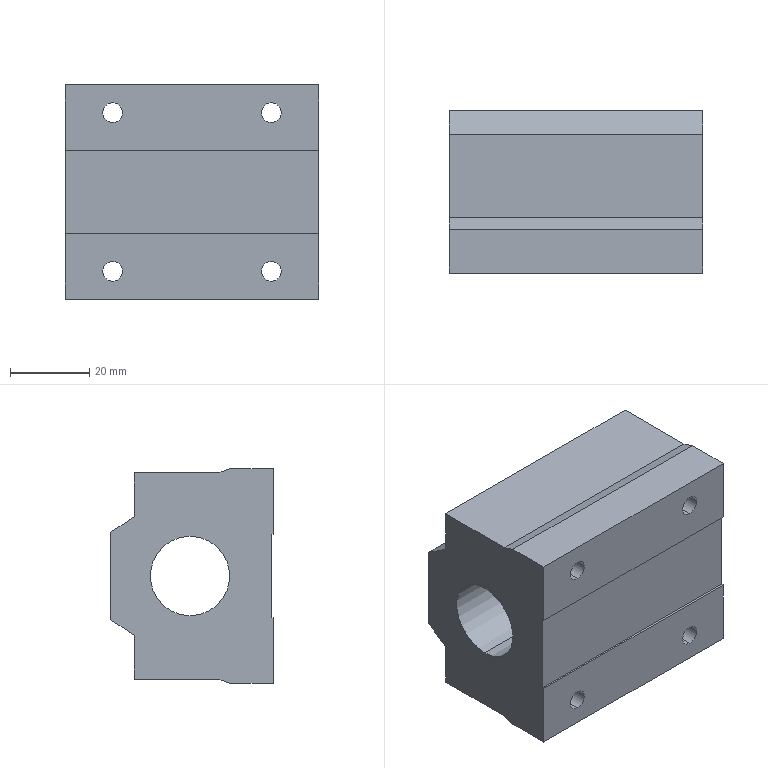Part | STEP file | Linear bearing LHBB-MX 20 | 1 solid | 28 faces | box 64 x 41 x 54 mm | volume 104537 mm3 | plane 18 | cylinder 10 | commonest cylinder face diameters 5 x8 20 x2